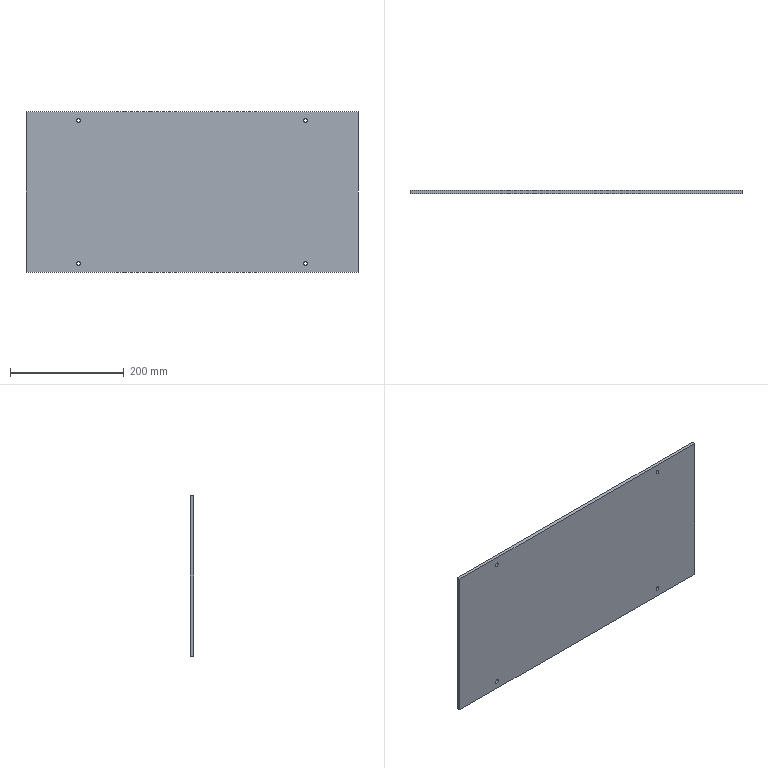Part | SolidWorks | features BaseBody 1 | 1 solid | 14 faces | box 585 x 6 x 282 mm | volume 988896 mm3 | cylinder 8 | plane 6 | commonest cylinder face diameters 7 x8
STEP:
#1=CARTESIAN_POINT('',(200.,0.,-129.5));
#2=VERTEX_POINT('',#1);
#3=CARTESIAN_POINT('',(200.,0.,-122.5));
#4=VERTEX_POINT('',#3);
#5=CARTESIAN_POINT('',(200.,0.,-126.));
#6=DIRECTION('',(0.,1.,0.));
#7=DIRECTION('',(0.,0.,1.));
#8=AXIS2_PLACEMENT_3D('',#5,#6,#7);
#9=CIRCLE('',#8,3.5);
#10=EDGE_CURVE('',#2,#4,#9,.T.);
#11=ORIENTED_EDGE('',*,*,#10,.F.);
#12=CARTESIAN_POINT('',(200.,6.,-129.5));
#13=VERTEX_POINT('',#12);
#14=CARTESIAN_POINT('',(200.,0.,-129.5));
#15=DIRECTION('',(0.,1.,0.));
#16=VECTOR('',#15,1000.);
#17=LINE('',#14,#16);
#18=EDGE_CURVE('',#2,#13,#17,.T.);
#19=ORIENTED_EDGE('',*,*,#18,.T.);
#20=CARTESIAN_POINT('',(200.,6.,-122.5));
#21=VERTEX_POINT('',#20);
#22=CARTESIAN_POINT('',(200.,6.,-126.));
#23=DIRECTION('',(0.,1.,0.));
#24=DIRECTION('',(0.,0.,1.));
#25=AXIS2_PLACEMENT_3D('',#22,#23,#24);
#26=CIRCLE('',#25,3.5);
#27=EDGE_CURVE('',#13,#21,#26,.T.);
#28=ORIENTED_EDGE('',*,*,#27,.T.);
#29=CARTESIAN_POINT('',(200.,0.,-122.5));
#30=DIRECTION('',(0.,1.,0.));
#31=VECTOR('',#30,1000.);
#32=LINE('',#29,#31);
#33=EDGE_CURVE('',#4,#21,#32,.T.);
#34=ORIENTED_EDGE('',*,*,#33,.F.);
#35=EDGE_LOOP('',(#11,#19,#28,#34));
#36=FACE_OUTER_BOUND('',#35,.T.);
#37=CARTESIAN_POINT('',(200.,0.,-126.));
#38=DIRECTION('',(0.,1.,0.));
#39=DIRECTION('',(0.,0.,1.));
#40=AXIS2_PLACEMENT_3D('',#37,#38,#39);
#41=CYLINDRICAL_SURFACE('',#40,3.5);
#42=ADVANCED_FACE('',(#36),#41,.F.);
#43=CARTESIAN_POINT('',(200.,0.,129.5));
#44=VERTEX_POINT('',#43);
#45=CARTESIAN_POINT('',(200.,0.,122.5));
#46=VERTEX_POINT('',#45);
#47=CARTESIAN_POINT('',(200.,0.,126.));
#48=DIRECTION('',(0.,-1.,0.));
#49=DIRECTION('',(0.,0.,-1.));
#50=AXIS2_PLACEMENT_3D('',#47,#48,#49);
#51=CIRCLE('',#50,3.5);
#52=EDGE_CURVE('',#44,#46,#51,.T.);
#53=ORIENTED_EDGE('',*,*,#52,.T.);
#54=CARTESIAN_POINT('',(200.,6.,122.5));
#55=VERTEX_POINT('',#54);
#56=CARTESIAN_POINT('',(200.,0.,122.5));
#57=DIRECTION('',(0.,1.,0.));
#58=VECTOR('',#57,1000.);
#59=LINE('',#56,#58);
#60=EDGE_CURVE('',#46,#55,#59,.T.);
#61=ORIENTED_EDGE('',*,*,#60,.T.);
#62=CARTESIAN_POINT('',(200.,6.,129.5));
#63=VERTEX_POINT('',#62);
#64=CARTESIAN_POINT('',(200.,6.,126.));
#65=DIRECTION('',(0.,-1.,0.));
#66=DIRECTION('',(0.,0.,-1.));
#67=AXIS2_PLACEMENT_3D('',#64,#65,#66);
#68=CIRCLE('',#67,3.5);
#69=EDGE_CURVE('',#63,#55,#68,.T.);
#70=ORIENTED_EDGE('',*,*,#69,.F.);
#71=CARTESIAN_POINT('',(200.,0.,129.5));
#72=DIRECTION('',(0.,1.,0.));
#73=VECTOR('',#72,1000.);
#74=LINE('',#71,#73);
#75=EDGE_CURVE('',#44,#63,#74,.T.);
#76=ORIENTED_EDGE('',*,*,#75,.F.);
#77=EDGE_LOOP('',(#53,#61,#70,#76));
#78=FACE_OUTER_BOUND('',#77,.T.);
#79=CARTESIAN_POINT('',(200.,0.,126.));
#80=DIRECTION('',(0.,1.,0.));
#81=DIRECTION('',(0.,0.,1.));
#82=AXIS2_PLACEMENT_3D('',#79,#80,#81);
#83=CYLINDRICAL_SURFACE('',#82,3.5);
#84=ADVANCED_FACE('',(#78),#83,.F.);
#85=CARTESIAN_POINT('',(-200.,0.,129.5));
#86=VERTEX_POINT('',#85);
#87=CARTESIAN_POINT('',(-200.,0.,122.5));
#88=VERTEX_POINT('',#87);
#89=CARTESIAN_POINT('',(-200.,0.,126.));
#90=DIRECTION('',(0.,-1.,0.));
#91=DIRECTION('',(0.,0.,-1.));
#92=AXIS2_PLACEMENT_3D('',#89,#90,#91);
#93=CIRCLE('',#92,3.5);
#94=EDGE_CURVE('',#86,#88,#93,.T.);
#95=ORIENTED_EDGE('',*,*,#94,.T.);
#96=CARTESIAN_POINT('',(-200.,6.,122.5));
#97=VERTEX_POINT('',#96);
#98=CARTESIAN_POINT('',(-200.,0.,122.5));
#99=DIRECTION('',(0.,1.,0.));
#100=VECTOR('',#99,1000.);
#101=LINE('',#98,#100);
#102=EDGE_CURVE('',#88,#97,#101,.T.);
#103=ORIENTED_EDGE('',*,*,#102,.T.);
#104=CARTESIAN_POINT('',(-200.,6.,129.5));
#105=VERTEX_POINT('',#104);
#106=CARTESIAN_POINT('',(-200.,6.,126.));
#107=DIRECTION('',(0.,-1.,0.));
#108=DIRECTION('',(0.,0.,-1.));
#109=AXIS2_PLACEMENT_3D('',#106,#107,#108);
#110=CIRCLE('',#109,3.5);
#111=EDGE_CURVE('',#105,#97,#110,.T.);
#112=ORIENTED_EDGE('',*,*,#111,.F.);
#113=CARTESIAN_POINT('',(-200.,0.,129.5));
#114=DIRECTION('',(0.,1.,0.));
#115=VECTOR('',#114,1000.);
#116=LINE('',#113,#115);
#117=EDGE_CURVE('',#86,#105,#116,.T.);
#118=ORIENTED_EDGE('',*,*,#117,.F.);
#119=EDGE_LOOP('',(#95,#103,#112,#118));
#120=FACE_OUTER_BOUND('',#119,.T.);
#121=CARTESIAN_POINT('',(-200.,0.,126.));
#122=DIRECTION('',(0.,1.,0.));
#123=DIRECTION('',(0.,0.,1.));
#124=AXIS2_PLACEMENT_3D('',#121,#122,#123);
#125=CYLINDRICAL_SURFACE('',#124,3.5);
#126=ADVANCED_FACE('',(#120),#125,.F.);
#127=CARTESIAN_POINT('',(-200.,0.,-129.5));
#128=VERTEX_POINT('',#127);
#129=CARTESIAN_POINT('',(-200.,0.,-122.5));
#130=VERTEX_POINT('',#129);
#131=CARTESIAN_POINT('',(-200.,0.,-126.));
#132=DIRECTION('',(0.,1.,0.));
#133=DIRECTION('',(0.,0.,1.));
#134=AXIS2_PLACEMENT_3D('',#131,#132,#133);
#135=CIRCLE('',#134,3.5);
#136=EDGE_CURVE('',#128,#130,#135,.T.);
#137=ORIENTED_EDGE('',*,*,#136,.F.);
#138=CARTESIAN_POINT('',(-200.,6.,-129.5));
#139=VERTEX_POINT('',#138);
#140=CARTESIAN_POINT('',(-200.,0.,-129.5));
#141=DIRECTION('',(0.,1.,0.));
#142=VECTOR('',#141,1000.);
#143=LINE('',#140,#142);
#144=EDGE_CURVE('',#128,#139,#143,.T.);
#145=ORIENTED_EDGE('',*,*,#144,.T.);
#146=CARTESIAN_POINT('',(-200.,6.,-122.5));
#147=VERTEX_POINT('',#146);
#148=CARTESIAN_POINT('',(-200.,6.,-126.));
#149=DIRECTION('',(0.,1.,0.));
#150=DIRECTION('',(0.,0.,1.));
#151=AXIS2_PLACEMENT_3D('',#148,#149,#150);
#152=CIRCLE('',#151,3.5);
#153=EDGE_CURVE('',#139,#147,#152,.T.);
#154=ORIENTED_EDGE('',*,*,#153,.T.);
#155=CARTESIAN_POINT('',(-200.,0.,-122.5));
#156=DIRECTION('',(0.,1.,0.));
#157=VECTOR('',#156,1000.);
#158=LINE('',#155,#157);
#159=EDGE_CURVE('',#130,#147,#158,.T.);
#160=ORIENTED_EDGE('',*,*,#159,.F.);
#161=EDGE_LOOP('',(#137,#145,#154,#160));
#162=FACE_OUTER_BOUND('',#161,.T.);
#163=CARTESIAN_POINT('',(-200.,0.,-126.));
#164=DIRECTION('',(0.,1.,0.));
#165=DIRECTION('',(0.,0.,1.));
#166=AXIS2_PLACEMENT_3D('',#163,#164,#165);
#167=CYLINDRICAL_SURFACE('',#166,3.5);
#168=ADVANCED_FACE('',(#162),#167,.F.);
#169=CARTESIAN_POINT('',(-292.5,0.,141.));
#170=VERTEX_POINT('',#169);
#171=CARTESIAN_POINT('',(292.5,0.,141.));
#172=VERTEX_POINT('',#171);
#173=CARTESIAN_POINT('',(-292.5,0.,141.));
#174=DIRECTION('',(1.,0.,0.));
#175=VECTOR('',#174,1000.);
#176=LINE('',#173,#175);
#177=EDGE_CURVE('',#170,#172,#176,.T.);
#178=ORIENTED_EDGE('',*,*,#177,.T.);
#179=CARTESIAN_POINT('',(292.5,6.,141.));
#180=VERTEX_POINT('',#179);
#181=CARTESIAN_POINT('',(292.5,6.,141.));
#182=DIRECTION('',(0.,-1.,0.));
#183=VECTOR('',#182,1000.);
#184=LINE('',#181,#183);
#185=EDGE_CURVE('',#180,#172,#184,.T.);
#186=ORIENTED_EDGE('',*,*,#185,.F.);
#187=CARTESIAN_POINT('',(-292.5,6.,141.));
#188=VERTEX_POINT('',#187);
#189=CARTESIAN_POINT('',(-292.5,6.,141.));
#190=DIRECTION('',(1.,0.,0.));
#191=VECTOR('',#190,1000.);
#192=LINE('',#189,#191);
#193=EDGE_CURVE('',#188,#180,#192,.T.);
#194=ORIENTED_EDGE('',*,*,#193,.F.);
#195=CARTESIAN_POINT('',(-292.5,6.,141.));
#196=DIRECTION('',(0.,-1.,0.));
#197=VECTOR('',#196,1000.);
#198=LINE('',#195,#197);
#199=EDGE_CURVE('',#188,#170,#198,.T.);
#200=ORIENTED_EDGE('',*,*,#199,.T.);
#201=EDGE_LOOP('',(#178,#186,#194,#200));
#202=FACE_OUTER_BOUND('',#201,.T.);
#203=CARTESIAN_POINT('',(-292.5,6.,141.));
#204=DIRECTION('',(0.,0.,-1.));
#205=DIRECTION('',(0.,-1.,0.));
#206=AXIS2_PLACEMENT_3D('',#203,#204,#205);
#207=PLANE('',#206);
#208=ADVANCED_FACE('',(#202),#207,.F.);
#209=CARTESIAN_POINT('',(-292.5,0.,-141.));
#210=VERTEX_POINT('',#209);
#211=CARTESIAN_POINT('',(-292.5,0.,141.));
#212=DIRECTION('',(0.,0.,1.));
#213=VECTOR('',#212,1000.);
#214=LINE('',#211,#213);
#215=EDGE_CURVE('',#210,#170,#214,.T.);
#216=ORIENTED_EDGE('',*,*,#215,.T.);
#217=ORIENTED_EDGE('',*,*,#199,.F.);
#218=CARTESIAN_POINT('',(-292.5,6.,-141.));
#219=VERTEX_POINT('',#218);
#220=CARTESIAN_POINT('',(-292.5,6.,141.));
#221=DIRECTION('',(0.,0.,1.));
#222=VECTOR('',#221,1000.);
#223=LINE('',#220,#222);
#224=EDGE_CURVE('',#219,#188,#223,.T.);
#225=ORIENTED_EDGE('',*,*,#224,.F.);
#226=CARTESIAN_POINT('',(-292.5,6.,-141.));
#227=DIRECTION('',(0.,-1.,0.));
#228=VECTOR('',#227,1000.);
#229=LINE('',#226,#228);
#230=EDGE_CURVE('',#219,#210,#229,.T.);
#231=ORIENTED_EDGE('',*,*,#230,.T.);
#232=EDGE_LOOP('',(#216,#217,#225,#231));
#233=FACE_OUTER_BOUND('',#232,.T.);
#234=CARTESIAN_POINT('',(-292.5,6.,141.));
#235=DIRECTION('',(1.,0.,0.));
#236=DIRECTION('',(0.,1.,0.));
#237=AXIS2_PLACEMENT_3D('',#234,#235,#236);
#238=PLANE('',#237);
#239=ADVANCED_FACE('',(#233),#238,.F.);
#240=CARTESIAN_POINT('',(292.5,0.,-141.));
#241=VERTEX_POINT('',#240);
#242=CARTESIAN_POINT('',(-292.5,0.,-141.));
#243=DIRECTION('',(-1.,0.,0.));
#244=VECTOR('',#243,1000.);
#245=LINE('',#242,#244);
#246=EDGE_CURVE('',#241,#210,#245,.T.);
#247=ORIENTED_EDGE('',*,*,#246,.T.);
#248=ORIENTED_EDGE('',*,*,#230,.F.);
#249=CARTESIAN_POINT('',(292.5,6.,-141.));
#250=VERTEX_POINT('',#249);
#251=CARTESIAN_POINT('',(-292.5,6.,-141.));
#252=DIRECTION('',(-1.,0.,0.));
#253=VECTOR('',#252,1000.);
#254=LINE('',#251,#253);
#255=EDGE_CURVE('',#250,#219,#254,.T.);
#256=ORIENTED_EDGE('',*,*,#255,.F.);
#257=CARTESIAN_POINT('',(292.5,6.,-141.));
#258=DIRECTION('',(0.,-1.,0.));
#259=VECTOR('',#258,1000.);
#260=LINE('',#257,#259);
#261=EDGE_CURVE('',#250,#241,#260,.T.);
#262=ORIENTED_EDGE('',*,*,#261,.T.);
#263=EDGE_LOOP('',(#247,#248,#256,#262));
#264=FACE_OUTER_BOUND('',#263,.T.);
#265=CARTESIAN_POINT('',(-292.5,6.,-141.));
#266=DIRECTION('',(0.,0.,1.));
#267=DIRECTION('',(1.,0.,0.));
#268=AXIS2_PLACEMENT_3D('',#265,#266,#267);
#269=PLANE('',#268);
#270=ADVANCED_FACE('',(#264),#269,.F.);
#271=CARTESIAN_POINT('',(292.5,0.,141.));
#272=DIRECTION('',(0.,0.,-1.));
#273=VECTOR('',#272,1000.);
#274=LINE('',#271,#273);
#275=EDGE_CURVE('',#172,#241,#274,.T.);
#276=ORIENTED_EDGE('',*,*,#275,.T.);
#277=ORIENTED_EDGE('',*,*,#261,.F.);
#278=CARTESIAN_POINT('',(292.5,6.,141.));
#279=DIRECTION('',(0.,0.,-1.));
#280=VECTOR('',#279,1000.);
#281=LINE('',#278,#280);
#282=EDGE_CURVE('',#180,#250,#281,.T.);
#283=ORIENTED_EDGE('',*,*,#282,.F.);
#284=ORIENTED_EDGE('',*,*,#185,.T.);
#285=EDGE_LOOP('',(#276,#277,#283,#284));
#286=FACE_OUTER_BOUND('',#285,.T.);
#287=CARTESIAN_POINT('',(292.5,6.,141.));
#288=DIRECTION('',(-1.,0.,0.));
#289=DIRECTION('',(0.,0.,1.));
#290=AXIS2_PLACEMENT_3D('',#287,#288,#289);
#291=PLANE('',#290);
#292=ADVANCED_FACE('',(#286),#291,.F.);
#293=ORIENTED_EDGE('',*,*,#52,.F.);
#294=CARTESIAN_POINT('',(200.,0.,126.));
#295=DIRECTION('',(0.,-1.,0.));
#296=DIRECTION('',(0.,0.,-1.));
#297=AXIS2_PLACEMENT_3D('',#294,#295,#296);
#298=CIRCLE('',#297,3.5);
#299=EDGE_CURVE('',#46,#44,#298,.T.);
#300=ORIENTED_EDGE('',*,*,#299,.F.);
#301=EDGE_LOOP('',(#293,#300));
#302=FACE_BOUND('',#301,.T.);
#303=CARTESIAN_POINT('',(-200.,0.,-126.));
#304=DIRECTION('',(0.,1.,0.));
#305=DIRECTION('',(0.,0.,1.));
#306=AXIS2_PLACEMENT_3D('',#303,#304,#305);
#307=CIRCLE('',#306,3.5);
#308=EDGE_CURVE('',#130,#128,#307,.T.);
#309=ORIENTED_EDGE('',*,*,#308,.T.);
#310=ORIENTED_EDGE('',*,*,#136,.T.);
#311=EDGE_LOOP('',(#309,#310));
#312=FACE_BOUND('',#311,.T.);
#313=ORIENTED_EDGE('',*,*,#94,.F.);
#314=CARTESIAN_POINT('',(-200.,0.,126.));
#315=DIRECTION('',(0.,-1.,0.));
#316=DIRECTION('',(0.,0.,-1.));
#317=AXIS2_PLACEMENT_3D('',#314,#315,#316);
#318=CIRCLE('',#317,3.5);
#319=EDGE_CURVE('',#88,#86,#318,.T.);
#320=ORIENTED_EDGE('',*,*,#319,.F.);
#321=EDGE_LOOP('',(#313,#320));
#322=FACE_BOUND('',#321,.T.);
#323=CARTESIAN_POINT('',(200.,0.,-126.));
#324=DIRECTION('',(0.,1.,0.));
#325=DIRECTION('',(0.,0.,1.));
#326=AXIS2_PLACEMENT_3D('',#323,#324,#325);
#327=CIRCLE('',#326,3.5);
#328=EDGE_CURVE('',#4,#2,#327,.T.);
#329=ORIENTED_EDGE('',*,*,#328,.T.);
#330=ORIENTED_EDGE('',*,*,#10,.T.);
#331=EDGE_LOOP('',(#329,#330));
#332=FACE_BOUND('',#331,.T.);
#333=ORIENTED_EDGE('',*,*,#275,.F.);
#334=ORIENTED_EDGE('',*,*,#177,.F.);
#335=ORIENTED_EDGE('',*,*,#215,.F.);
#336=ORIENTED_EDGE('',*,*,#246,.F.);
#337=EDGE_LOOP('',(#333,#334,#335,#336));
#338=FACE_OUTER_BOUND('',#337,.T.);
#339=CARTESIAN_POINT('',(0.,0.,0.));
#340=DIRECTION('',(0.,-1.,0.));
#341=DIRECTION('',(0.,0.,-1.));
#342=AXIS2_PLACEMENT_3D('',#339,#340,#341);
#343=PLANE('',#342);
#344=ADVANCED_FACE('',(#302,#312,#322,#332,#338),#343,.T.);
#345=ORIENTED_EDGE('',*,*,#69,.T.);
#346=CARTESIAN_POINT('',(200.,6.,126.));
#347=DIRECTION('',(0.,-1.,0.));
#348=DIRECTION('',(0.,0.,-1.));
#349=AXIS2_PLACEMENT_3D('',#346,#347,#348);
#350=CIRCLE('',#349,3.5);
#351=EDGE_CURVE('',#55,#63,#350,.T.);
#352=ORIENTED_EDGE('',*,*,#351,.T.);
#353=EDGE_LOOP('',(#345,#352));
#354=FACE_BOUND('',#353,.T.);
#355=CARTESIAN_POINT('',(-200.,6.,-126.));
#356=DIRECTION('',(0.,1.,0.));
#357=DIRECTION('',(0.,0.,1.));
#358=AXIS2_PLACEMENT_3D('',#355,#356,#357);
#359=CIRCLE('',#358,3.5);
#360=EDGE_CURVE('',#147,#139,#359,.T.);
#361=ORIENTED_EDGE('',*,*,#360,.F.);
#362=ORIENTED_EDGE('',*,*,#153,.F.);
#363=EDGE_LOOP('',(#361,#362));
#364=FACE_BOUND('',#363,.T.);
#365=ORIENTED_EDGE('',*,*,#111,.T.);
#366=CARTESIAN_POINT('',(-200.,6.,126.));
#367=DIRECTION('',(0.,-1.,0.));
#368=DIRECTION('',(0.,0.,-1.));
#369=AXIS2_PLACEMENT_3D('',#366,#367,#368);
#370=CIRCLE('',#369,3.5);
#371=EDGE_CURVE('',#97,#105,#370,.T.);
#372=ORIENTED_EDGE('',*,*,#371,.T.);
#373=EDGE_LOOP('',(#365,#372));
#374=FACE_BOUND('',#373,.T.);
#375=CARTESIAN_POINT('',(200.,6.,-126.));
#376=DIRECTION('',(0.,1.,0.));
#377=DIRECTION('',(0.,0.,1.));
#378=AXIS2_PLACEMENT_3D('',#375,#376,#377);
#379=CIRCLE('',#378,3.5);
#380=EDGE_CURVE('',#21,#13,#379,.T.);
#381=ORIENTED_EDGE('',*,*,#380,.F.);
#382=ORIENTED_EDGE('',*,*,#27,.F.);
#383=EDGE_LOOP('',(#381,#382));
#384=FACE_BOUND('',#383,.T.);
#385=ORIENTED_EDGE('',*,*,#282,.T.);
#386=ORIENTED_EDGE('',*,*,#255,.T.);
#387=ORIENTED_EDGE('',*,*,#224,.T.);
#388=ORIENTED_EDGE('',*,*,#193,.T.);
#389=EDGE_LOOP('',(#385,#386,#387,#388));
#390=FACE_OUTER_BOUND('',#389,.T.);
#391=CARTESIAN_POINT('',(0.,6.,0.));
#392=DIRECTION('',(0.,-1.,0.));
#393=DIRECTION('',(0.,0.,-1.));
#394=AXIS2_PLACEMENT_3D('',#391,#392,#393);
#395=PLANE('',#394);
#396=ADVANCED_FACE('',(#354,#364,#374,#384,#390),#395,.F.);
#397=ORIENTED_EDGE('',*,*,#144,.F.);
#398=ORIENTED_EDGE('',*,*,#308,.F.);
#399=ORIENTED_EDGE('',*,*,#159,.T.);
#400=ORIENTED_EDGE('',*,*,#360,.T.);
#401=EDGE_LOOP('',(#397,#398,#399,#400));
#402=FACE_OUTER_BOUND('',#401,.T.);
#403=CARTESIAN_POINT('',(-200.,0.,-126.));
#404=DIRECTION('',(0.,1.,0.));
#405=DIRECTION('',(0.,0.,1.));
#406=AXIS2_PLACEMENT_3D('',#403,#404,#405);
#407=CYLINDRICAL_SURFACE('',#406,3.5);
#408=ADVANCED_FACE('',(#402),#407,.F.);
#409=ORIENTED_EDGE('',*,*,#102,.F.);
#410=ORIENTED_EDGE('',*,*,#319,.T.);
#411=ORIENTED_EDGE('',*,*,#117,.T.);
#412=ORIENTED_EDGE('',*,*,#371,.F.);
#413=EDGE_LOOP('',(#409,#410,#411,#412));
#414=FACE_OUTER_BOUND('',#413,.T.);
#415=CARTESIAN_POINT('',(-200.,0.,126.));
#416=DIRECTION('',(0.,1.,0.));
#417=DIRECTION('',(0.,0.,1.));
#418=AXIS2_PLACEMENT_3D('',#415,#416,#417);
#419=CYLINDRICAL_SURFACE('',#418,3.5);
#420=ADVANCED_FACE('',(#414),#419,.F.);
#421=ORIENTED_EDGE('',*,*,#60,.F.);
#422=ORIENTED_EDGE('',*,*,#299,.T.);
#423=ORIENTED_EDGE('',*,*,#75,.T.);
#424=ORIENTED_EDGE('',*,*,#351,.F.);
#425=EDGE_LOOP('',(#421,#422,#423,#424));
#426=FACE_OUTER_BOUND('',#425,.T.);
#427=CARTESIAN_POINT('',(200.,0.,126.));
#428=DIRECTION('',(0.,1.,0.));
#429=DIRECTION('',(0.,0.,1.));
#430=AXIS2_PLACEMENT_3D('',#427,#428,#429);
#431=CYLINDRICAL_SURFACE('',#430,3.5);
#432=ADVANCED_FACE('',(#426),#431,.F.);
#433=ORIENTED_EDGE('',*,*,#18,.F.);
#434=ORIENTED_EDGE('',*,*,#328,.F.);
#435=ORIENTED_EDGE('',*,*,#33,.T.);
#436=ORIENTED_EDGE('',*,*,#380,.T.);
#437=EDGE_LOOP('',(#433,#434,#435,#436));
#438=FACE_OUTER_BOUND('',#437,.T.);
#439=CARTESIAN_POINT('',(200.,0.,-126.));
#440=DIRECTION('',(0.,1.,0.));
#441=DIRECTION('',(0.,0.,1.));
#442=AXIS2_PLACEMENT_3D('',#439,#440,#441);
#443=CYLINDRICAL_SURFACE('',#442,3.5);
#444=ADVANCED_FACE('',(#438),#443,.F.);
#445=CLOSED_SHELL('',(#42,#84,#126,#168,#208,#239,#270,#292,#344,#396,#408,#420,#432,#444));
#446=MANIFOLD_SOLID_BREP('',#445);
#447=CARTESIAN_POINT('',(0.,0.,0.));
#448=DIRECTION('',(0.,0.,1.));
#449=DIRECTION('',(1.,0.,0.));
#450=AXIS2_PLACEMENT_3D('',#447,#448,#449);
#451=(LENGTH_UNIT()NAMED_UNIT(*)SI_UNIT(.MILLI.,.METRE.));
#452=UNCERTAINTY_MEASURE_WITH_UNIT(LENGTH_MEASURE(0.00001),#451,'','');
#453=(NAMED_UNIT(*)PLANE_ANGLE_UNIT()SI_UNIT($,.RADIAN.));
#454=(NAMED_UNIT(*)SI_UNIT($,.STERADIAN.)SOLID_ANGLE_UNIT());
#455=(GEOMETRIC_REPRESENTATION_CONTEXT(3)GLOBAL_UNCERTAINTY_ASSIGNED_CONTEXT((#452))GLOBAL_UNIT_ASSIGNED_CONTEXT((#451,#453,#454))REPRESENTATION_CONTEXT('',''));
#456=ADVANCED_BREP_SHAPE_REPRESENTATION('',(#446,#450),#455);